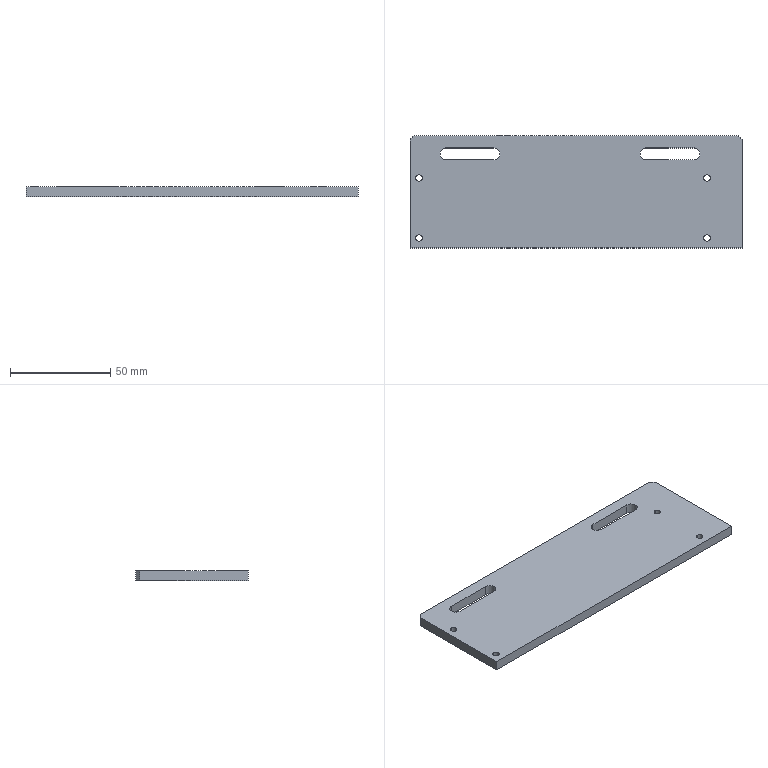Part | NX | features solid 2 | 1 solid | 24 faces | box 166 x 56 x 5 mm | volume 44572 mm3 | plane 12 | cylinder 12 | commonest cylinder face diameters 3.242 x8 6 x4
STEP:
#1=CARTESIAN_POINT('',(-350.,-1555.5,1295.));
#2=VERTEX_POINT('',#1);
#3=CARTESIAN_POINT('',(-350.,-1555.5,1300.));
#4=VERTEX_POINT('',#3);
#5=CARTESIAN_POINT('',(-350.,-1555.5,1300.));
#6=DIRECTION('',(0.,0.,1.));
#7=VECTOR('',#6,1000.);
#8=LINE('',#5,#7);
#9=EDGE_CURVE('',#2,#4,#8,.T.);
#10=ORIENTED_EDGE('',*,*,#9,.T.);
#11=CARTESIAN_POINT('',(-516.,-1555.5,1300.));
#12=VERTEX_POINT('',#11);
#13=CARTESIAN_POINT('',(-433.,-1555.5,1300.));
#14=DIRECTION('',(1.,0.,0.));
#15=VECTOR('',#14,1000.);
#16=LINE('',#13,#15);
#17=EDGE_CURVE('',#12,#4,#16,.T.);
#18=ORIENTED_EDGE('',*,*,#17,.F.);
#19=CARTESIAN_POINT('',(-516.,-1555.5,1295.));
#20=VERTEX_POINT('',#19);
#21=CARTESIAN_POINT('',(-516.,-1555.5,1300.));
#22=DIRECTION('',(0.,0.,1.));
#23=VECTOR('',#22,1000.);
#24=LINE('',#21,#23);
#25=EDGE_CURVE('',#20,#12,#24,.T.);
#26=ORIENTED_EDGE('',*,*,#25,.F.);
#27=CARTESIAN_POINT('',(-433.,-1555.5,1295.));
#28=DIRECTION('',(1.,0.,0.));
#29=VECTOR('',#28,1000.);
#30=LINE('',#27,#29);
#31=EDGE_CURVE('',#20,#2,#30,.T.);
#32=ORIENTED_EDGE('',*,*,#31,.T.);
#33=EDGE_LOOP('',(#10,#18,#26,#32));
#34=FACE_BOUND('',#33,.T.);
#35=CARTESIAN_POINT('',(-433.,-1555.5,1300.));
#36=DIRECTION('',(0.,-1.,0.));
#37=DIRECTION('',(0.,0.,-1.));
#38=AXIS2_PLACEMENT_3D('',#35,#36,#37);
#39=PLANE('',#38);
#40=ADVANCED_FACE('',(#34),#39,.T.);
#41=CARTESIAN_POINT('',(-367.5,-1518.879,1295.));
#42=VERTEX_POINT('',#41);
#43=CARTESIAN_POINT('',(-367.5,-1518.879,1300.));
#44=VERTEX_POINT('',#43);
#45=CARTESIAN_POINT('',(-367.5,-1518.879,1478.057));
#46=DIRECTION('',(0.,0.,-1.));
#47=VECTOR('',#46,1000.);
#48=LINE('',#45,#47);
#49=EDGE_CURVE('',#42,#44,#48,.F.);
#50=ORIENTED_EDGE('',*,*,#49,.T.);
#51=CARTESIAN_POINT('',(-367.5,-1522.121,1300.));
#52=VERTEX_POINT('',#51);
#53=CARTESIAN_POINT('',(-367.5,-1520.5,1300.));
#54=DIRECTION('',(0.,0.,1.));
#55=DIRECTION('',(0.,1.,0.));
#56=AXIS2_PLACEMENT_3D('',#53,#54,#55);
#57=CIRCLE('',#56,1.621);
#58=EDGE_CURVE('',#44,#52,#57,.T.);
#59=ORIENTED_EDGE('',*,*,#58,.T.);
#60=CARTESIAN_POINT('',(-367.5,-1522.121,1295.));
#61=VERTEX_POINT('',#60);
#62=CARTESIAN_POINT('',(-367.5,-1522.121,1478.057));
#63=DIRECTION('',(0.,0.,-1.));
#64=VECTOR('',#63,1000.);
#65=LINE('',#62,#64);
#66=EDGE_CURVE('',#52,#61,#65,.T.);
#67=ORIENTED_EDGE('',*,*,#66,.T.);
#68=CARTESIAN_POINT('',(-367.5,-1520.5,1295.));
#69=DIRECTION('',(0.,0.,-1.));
#70=DIRECTION('',(-1.,0.,0.));
#71=AXIS2_PLACEMENT_3D('',#68,#69,#70);
#72=CIRCLE('',#71,1.621);
#73=EDGE_CURVE('',#61,#42,#72,.T.);
#74=ORIENTED_EDGE('',*,*,#73,.T.);
#75=EDGE_LOOP('',(#50,#59,#67,#74));
#76=FACE_BOUND('',#75,.T.);
#77=CARTESIAN_POINT('',(-367.5,-1520.5,1478.057));
#78=DIRECTION('',(0.,0.,-1.));
#79=DIRECTION('',(0.,-1.,0.));
#80=AXIS2_PLACEMENT_3D('',#77,#78,#79);
#81=CYLINDRICAL_SURFACE('',#80,1.621);
#82=ADVANCED_FACE('',(#76),#81,.F.);
#83=CARTESIAN_POINT('',(-511.5,-1518.879,1295.));
#84=VERTEX_POINT('',#83);
#85=CARTESIAN_POINT('',(-511.5,-1518.879,1300.));
#86=VERTEX_POINT('',#85);
#87=CARTESIAN_POINT('',(-511.5,-1518.879,1478.057));
#88=DIRECTION('',(0.,0.,-1.));
#89=VECTOR('',#88,1000.);
#90=LINE('',#87,#89);
#91=EDGE_CURVE('',#84,#86,#90,.F.);
#92=ORIENTED_EDGE('',*,*,#91,.T.);
#93=CARTESIAN_POINT('',(-511.5,-1522.121,1300.));
#94=VERTEX_POINT('',#93);
#95=CARTESIAN_POINT('',(-511.5,-1520.5,1300.));
#96=DIRECTION('',(0.,0.,1.));
#97=DIRECTION('',(0.,1.,0.));
#98=AXIS2_PLACEMENT_3D('',#95,#96,#97);
#99=CIRCLE('',#98,1.621);
#100=EDGE_CURVE('',#86,#94,#99,.T.);
#101=ORIENTED_EDGE('',*,*,#100,.T.);
#102=CARTESIAN_POINT('',(-511.5,-1522.121,1295.));
#103=VERTEX_POINT('',#102);
#104=CARTESIAN_POINT('',(-511.5,-1522.121,1478.057));
#105=DIRECTION('',(0.,0.,-1.));
#106=VECTOR('',#105,1000.);
#107=LINE('',#104,#106);
#108=EDGE_CURVE('',#94,#103,#107,.T.);
#109=ORIENTED_EDGE('',*,*,#108,.T.);
#110=CARTESIAN_POINT('',(-511.5,-1520.5,1295.));
#111=DIRECTION('',(0.,0.,-1.));
#112=DIRECTION('',(-1.,0.,0.));
#113=AXIS2_PLACEMENT_3D('',#110,#111,#112);
#114=CIRCLE('',#113,1.621);
#115=EDGE_CURVE('',#103,#84,#114,.T.);
#116=ORIENTED_EDGE('',*,*,#115,.T.);
#117=EDGE_LOOP('',(#92,#101,#109,#116));
#118=FACE_BOUND('',#117,.T.);
#119=CARTESIAN_POINT('',(-511.5,-1520.5,1478.057));
#120=DIRECTION('',(0.,0.,-1.));
#121=DIRECTION('',(0.,-1.,0.));
#122=AXIS2_PLACEMENT_3D('',#119,#120,#121);
#123=CYLINDRICAL_SURFACE('',#122,1.621);
#124=ADVANCED_FACE('',(#118),#123,.F.);
#125=CARTESIAN_POINT('',(-511.5,-1548.879,1300.));
#126=VERTEX_POINT('',#125);
#127=CARTESIAN_POINT('',(-511.5,-1548.879,1295.));
#128=VERTEX_POINT('',#127);
#129=CARTESIAN_POINT('',(-511.5,-1548.879,1478.057));
#130=DIRECTION('',(0.,0.,-1.));
#131=VECTOR('',#130,1000.);
#132=LINE('',#129,#131);
#133=EDGE_CURVE('',#126,#128,#132,.T.);
#134=ORIENTED_EDGE('',*,*,#133,.F.);
#135=CARTESIAN_POINT('',(-511.5,-1552.121,1300.));
#136=VERTEX_POINT('',#135);
#137=CARTESIAN_POINT('',(-511.5,-1550.5,1300.));
#138=DIRECTION('',(0.,0.,1.));
#139=DIRECTION('',(0.,1.,0.));
#140=AXIS2_PLACEMENT_3D('',#137,#138,#139);
#141=CIRCLE('',#140,1.621);
#142=EDGE_CURVE('',#126,#136,#141,.T.);
#143=ORIENTED_EDGE('',*,*,#142,.T.);
#144=CARTESIAN_POINT('',(-511.5,-1552.121,1295.));
#145=VERTEX_POINT('',#144);
#146=CARTESIAN_POINT('',(-511.5,-1552.121,1478.057));
#147=DIRECTION('',(0.,0.,-1.));
#148=VECTOR('',#147,1000.);
#149=LINE('',#146,#148);
#150=EDGE_CURVE('',#145,#136,#149,.F.);
#151=ORIENTED_EDGE('',*,*,#150,.F.);
#152=CARTESIAN_POINT('',(-511.5,-1550.5,1295.));
#153=DIRECTION('',(0.,0.,-1.));
#154=DIRECTION('',(-1.,0.,0.));
#155=AXIS2_PLACEMENT_3D('',#152,#153,#154);
#156=CIRCLE('',#155,1.621);
#157=EDGE_CURVE('',#145,#128,#156,.T.);
#158=ORIENTED_EDGE('',*,*,#157,.T.);
#159=EDGE_LOOP('',(#134,#143,#151,#158));
#160=FACE_BOUND('',#159,.T.);
#161=CARTESIAN_POINT('',(-511.5,-1550.5,1478.057));
#162=DIRECTION('',(0.,0.,-1.));
#163=DIRECTION('',(0.,-1.,0.));
#164=AXIS2_PLACEMENT_3D('',#161,#162,#163);
#165=CYLINDRICAL_SURFACE('',#164,1.621);
#166=ADVANCED_FACE('',(#160),#165,.F.);
#167=CARTESIAN_POINT('',(-367.5,-1548.879,1300.));
#168=VERTEX_POINT('',#167);
#169=CARTESIAN_POINT('',(-367.5,-1548.879,1295.));
#170=VERTEX_POINT('',#169);
#171=CARTESIAN_POINT('',(-367.5,-1548.879,1478.057));
#172=DIRECTION('',(0.,0.,-1.));
#173=VECTOR('',#172,1000.);
#174=LINE('',#171,#173);
#175=EDGE_CURVE('',#168,#170,#174,.T.);
#176=ORIENTED_EDGE('',*,*,#175,.F.);
#177=CARTESIAN_POINT('',(-367.5,-1552.121,1300.));
#178=VERTEX_POINT('',#177);
#179=CARTESIAN_POINT('',(-367.5,-1550.5,1300.));
#180=DIRECTION('',(0.,0.,1.));
#181=DIRECTION('',(0.,1.,0.));
#182=AXIS2_PLACEMENT_3D('',#179,#180,#181);
#183=CIRCLE('',#182,1.621);
#184=EDGE_CURVE('',#168,#178,#183,.T.);
#185=ORIENTED_EDGE('',*,*,#184,.T.);
#186=CARTESIAN_POINT('',(-367.5,-1552.121,1295.));
#187=VERTEX_POINT('',#186);
#188=CARTESIAN_POINT('',(-367.5,-1552.121,1478.057));
#189=DIRECTION('',(0.,0.,-1.));
#190=VECTOR('',#189,1000.);
#191=LINE('',#188,#190);
#192=EDGE_CURVE('',#187,#178,#191,.F.);
#193=ORIENTED_EDGE('',*,*,#192,.F.);
#194=CARTESIAN_POINT('',(-367.5,-1550.5,1295.));
#195=DIRECTION('',(0.,0.,-1.));
#196=DIRECTION('',(-1.,0.,0.));
#197=AXIS2_PLACEMENT_3D('',#194,#195,#196);
#198=CIRCLE('',#197,1.621);
#199=EDGE_CURVE('',#187,#170,#198,.T.);
#200=ORIENTED_EDGE('',*,*,#199,.T.);
#201=EDGE_LOOP('',(#176,#185,#193,#200));
#202=FACE_BOUND('',#201,.T.);
#203=CARTESIAN_POINT('',(-367.5,-1550.5,1478.057));
#204=DIRECTION('',(0.,0.,-1.));
#205=DIRECTION('',(0.,-1.,0.));
#206=AXIS2_PLACEMENT_3D('',#203,#204,#205);
#207=CYLINDRICAL_SURFACE('',#206,1.621);
#208=ADVANCED_FACE('',(#202),#207,.F.);
#209=CARTESIAN_POINT('',(-398.,-1511.5,1300.));
#210=VERTEX_POINT('',#209);
#211=CARTESIAN_POINT('',(-374.,-1511.5,1300.));
#212=VERTEX_POINT('',#211);
#213=CARTESIAN_POINT('',(-433.,-1511.5,1300.));
#214=DIRECTION('',(1.,0.,0.));
#215=VECTOR('',#214,1000.);
#216=LINE('',#213,#215);
#217=EDGE_CURVE('',#210,#212,#216,.T.);
#218=ORIENTED_EDGE('',*,*,#217,.T.);
#219=CARTESIAN_POINT('',(-374.,-1511.5,1295.));
#220=VERTEX_POINT('',#219);
#221=CARTESIAN_POINT('',(-374.,-1511.5,1478.057));
#222=DIRECTION('',(0.,0.,-1.));
#223=VECTOR('',#222,1000.);
#224=LINE('',#221,#223);
#225=EDGE_CURVE('',#212,#220,#224,.T.);
#226=ORIENTED_EDGE('',*,*,#225,.T.);
#227=CARTESIAN_POINT('',(-398.,-1511.5,1295.));
#228=VERTEX_POINT('',#227);
#229=CARTESIAN_POINT('',(-374.,-1511.5,1295.));
#230=DIRECTION('',(-1.,0.,0.));
#231=VECTOR('',#230,1000.);
#232=LINE('',#229,#231);
#233=EDGE_CURVE('',#220,#228,#232,.T.);
#234=ORIENTED_EDGE('',*,*,#233,.T.);
#235=CARTESIAN_POINT('',(-398.,-1511.5,1478.057));
#236=DIRECTION('',(0.,0.,-1.));
#237=VECTOR('',#236,1000.);
#238=LINE('',#235,#237);
#239=EDGE_CURVE('',#210,#228,#238,.T.);
#240=ORIENTED_EDGE('',*,*,#239,.F.);
#241=EDGE_LOOP('',(#218,#226,#234,#240));
#242=FACE_BOUND('',#241,.T.);
#243=CARTESIAN_POINT('',(-374.,-1511.5,1478.057));
#244=DIRECTION('',(0.,-1.,0.));
#245=DIRECTION('',(0.,0.,-1.));
#246=AXIS2_PLACEMENT_3D('',#243,#244,#245);
#247=PLANE('',#246);
#248=ADVANCED_FACE('',(#242),#247,.F.);
#249=CARTESIAN_POINT('',(-374.,-1505.5,1300.));
#250=VERTEX_POINT('',#249);
#251=CARTESIAN_POINT('',(-374.,-1508.5,1300.));
#252=DIRECTION('',(0.,0.,1.));
#253=DIRECTION('',(0.,1.,0.));
#254=AXIS2_PLACEMENT_3D('',#251,#252,#253);
#255=CIRCLE('',#254,3.);
#256=EDGE_CURVE('',#212,#250,#255,.T.);
#257=ORIENTED_EDGE('',*,*,#256,.T.);
#258=CARTESIAN_POINT('',(-374.,-1505.5,1295.));
#259=VERTEX_POINT('',#258);
#260=CARTESIAN_POINT('',(-374.,-1505.5,1478.057));
#261=DIRECTION('',(0.,0.,-1.));
#262=VECTOR('',#261,1000.);
#263=LINE('',#260,#262);
#264=EDGE_CURVE('',#250,#259,#263,.T.);
#265=ORIENTED_EDGE('',*,*,#264,.T.);
#266=CARTESIAN_POINT('',(-374.,-1508.5,1295.));
#267=DIRECTION('',(0.,0.,-1.));
#268=DIRECTION('',(-1.,0.,0.));
#269=AXIS2_PLACEMENT_3D('',#266,#267,#268);
#270=CIRCLE('',#269,3.);
#271=EDGE_CURVE('',#259,#220,#270,.T.);
#272=ORIENTED_EDGE('',*,*,#271,.T.);
#273=ORIENTED_EDGE('',*,*,#225,.F.);
#274=EDGE_LOOP('',(#257,#265,#272,#273));
#275=FACE_BOUND('',#274,.T.);
#276=CARTESIAN_POINT('',(-374.,-1508.5,1478.057));
#277=DIRECTION('',(0.,0.,-1.));
#278=DIRECTION('',(0.,-1.,0.));
#279=AXIS2_PLACEMENT_3D('',#276,#277,#278);
#280=CYLINDRICAL_SURFACE('',#279,3.);
#281=ADVANCED_FACE('',(#275),#280,.F.);
#282=CARTESIAN_POINT('',(-398.,-1505.5,1300.));
#283=VERTEX_POINT('',#282);
#284=CARTESIAN_POINT('',(-433.,-1505.5,1300.));
#285=DIRECTION('',(-1.,0.,0.));
#286=VECTOR('',#285,1000.);
#287=LINE('',#284,#286);
#288=EDGE_CURVE('',#250,#283,#287,.T.);
#289=ORIENTED_EDGE('',*,*,#288,.T.);
#290=CARTESIAN_POINT('',(-398.,-1505.5,1295.));
#291=VERTEX_POINT('',#290);
#292=CARTESIAN_POINT('',(-398.,-1505.5,1478.057));
#293=DIRECTION('',(0.,0.,-1.));
#294=VECTOR('',#293,1000.);
#295=LINE('',#292,#294);
#296=EDGE_CURVE('',#283,#291,#295,.T.);
#297=ORIENTED_EDGE('',*,*,#296,.T.);
#298=CARTESIAN_POINT('',(-374.,-1505.5,1295.));
#299=DIRECTION('',(1.,0.,0.));
#300=VECTOR('',#299,1000.);
#301=LINE('',#298,#300);
#302=EDGE_CURVE('',#291,#259,#301,.T.);
#303=ORIENTED_EDGE('',*,*,#302,.T.);
#304=ORIENTED_EDGE('',*,*,#264,.F.);
#305=EDGE_LOOP('',(#289,#297,#303,#304));
#306=FACE_BOUND('',#305,.T.);
#307=CARTESIAN_POINT('',(-374.,-1505.5,1478.057));
#308=DIRECTION('',(0.,1.,0.));
#309=DIRECTION('',(1.,0.,0.));
#310=AXIS2_PLACEMENT_3D('',#307,#308,#309);
#311=PLANE('',#310);
#312=ADVANCED_FACE('',(#306),#311,.F.);
#313=CARTESIAN_POINT('',(-398.,-1508.5,1300.));
#314=DIRECTION('',(0.,0.,1.));
#315=DIRECTION('',(0.,1.,0.));
#316=AXIS2_PLACEMENT_3D('',#313,#314,#315);
#317=CIRCLE('',#316,3.);
#318=EDGE_CURVE('',#283,#210,#317,.T.);
#319=ORIENTED_EDGE('',*,*,#318,.T.);
#320=ORIENTED_EDGE('',*,*,#239,.T.);
#321=CARTESIAN_POINT('',(-398.,-1508.5,1295.));
#322=DIRECTION('',(0.,0.,-1.));
#323=DIRECTION('',(1.,0.,0.));
#324=AXIS2_PLACEMENT_3D('',#321,#322,#323);
#325=CIRCLE('',#324,3.);
#326=EDGE_CURVE('',#228,#291,#325,.T.);
#327=ORIENTED_EDGE('',*,*,#326,.T.);
#328=ORIENTED_EDGE('',*,*,#296,.F.);
#329=EDGE_LOOP('',(#319,#320,#327,#328));
#330=FACE_BOUND('',#329,.T.);
#331=CARTESIAN_POINT('',(-398.,-1508.5,1478.057));
#332=DIRECTION('',(0.,0.,-1.));
#333=DIRECTION('',(0.,-1.,0.));
#334=AXIS2_PLACEMENT_3D('',#331,#332,#333);
#335=CYLINDRICAL_SURFACE('',#334,3.);
#336=ADVANCED_FACE('',(#330),#335,.F.);
#337=CARTESIAN_POINT('',(-498.,-1511.5,1300.));
#338=VERTEX_POINT('',#337);
#339=CARTESIAN_POINT('',(-474.,-1511.5,1300.));
#340=VERTEX_POINT('',#339);
#341=CARTESIAN_POINT('',(-433.,-1511.5,1300.));
#342=DIRECTION('',(1.,0.,0.));
#343=VECTOR('',#342,1000.);
#344=LINE('',#341,#343);
#345=EDGE_CURVE('',#338,#340,#344,.T.);
#346=ORIENTED_EDGE('',*,*,#345,.T.);
#347=CARTESIAN_POINT('',(-474.,-1511.5,1295.));
#348=VERTEX_POINT('',#347);
#349=CARTESIAN_POINT('',(-474.,-1511.5,1478.057));
#350=DIRECTION('',(0.,0.,-1.));
#351=VECTOR('',#350,1000.);
#352=LINE('',#349,#351);
#353=EDGE_CURVE('',#340,#348,#352,.T.);
#354=ORIENTED_EDGE('',*,*,#353,.T.);
#355=CARTESIAN_POINT('',(-498.,-1511.5,1295.));
#356=VERTEX_POINT('',#355);
#357=CARTESIAN_POINT('',(-474.,-1511.5,1295.));
#358=DIRECTION('',(-1.,0.,0.));
#359=VECTOR('',#358,1000.);
#360=LINE('',#357,#359);
#361=EDGE_CURVE('',#348,#356,#360,.T.);
#362=ORIENTED_EDGE('',*,*,#361,.T.);
#363=CARTESIAN_POINT('',(-498.,-1511.5,1478.057));
#364=DIRECTION('',(0.,0.,-1.));
#365=VECTOR('',#364,1000.);
#366=LINE('',#363,#365);
#367=EDGE_CURVE('',#338,#356,#366,.T.);
#368=ORIENTED_EDGE('',*,*,#367,.F.);
#369=EDGE_LOOP('',(#346,#354,#362,#368));
#370=FACE_BOUND('',#369,.T.);
#371=CARTESIAN_POINT('',(-474.,-1511.5,1478.057));
#372=DIRECTION('',(0.,-1.,0.));
#373=DIRECTION('',(0.,0.,-1.));
#374=AXIS2_PLACEMENT_3D('',#371,#372,#373);
#375=PLANE('',#374);
#376=ADVANCED_FACE('',(#370),#375,.F.);
#377=CARTESIAN_POINT('',(-474.,-1505.5,1300.));
#378=VERTEX_POINT('',#377);
#379=CARTESIAN_POINT('',(-474.,-1508.5,1300.));
#380=DIRECTION('',(0.,0.,1.));
#381=DIRECTION('',(0.,1.,0.));
#382=AXIS2_PLACEMENT_3D('',#379,#380,#381);
#383=CIRCLE('',#382,3.);
#384=EDGE_CURVE('',#340,#378,#383,.T.);
#385=ORIENTED_EDGE('',*,*,#384,.T.);
#386=CARTESIAN_POINT('',(-474.,-1505.5,1295.));
#387=VERTEX_POINT('',#386);
#388=CARTESIAN_POINT('',(-474.,-1505.5,1478.057));
#389=DIRECTION('',(0.,0.,-1.));
#390=VECTOR('',#389,1000.);
#391=LINE('',#388,#390);
#392=EDGE_CURVE('',#378,#387,#391,.T.);
#393=ORIENTED_EDGE('',*,*,#392,.T.);
#394=CARTESIAN_POINT('',(-474.,-1508.5,1295.));
#395=DIRECTION('',(0.,0.,-1.));
#396=DIRECTION('',(-1.,0.,0.));
#397=AXIS2_PLACEMENT_3D('',#394,#395,#396);
#398=CIRCLE('',#397,3.);
#399=EDGE_CURVE('',#387,#348,#398,.T.);
#400=ORIENTED_EDGE('',*,*,#399,.T.);
#401=ORIENTED_EDGE('',*,*,#353,.F.);
#402=EDGE_LOOP('',(#385,#393,#400,#401));
#403=FACE_BOUND('',#402,.T.);
#404=CARTESIAN_POINT('',(-474.,-1508.5,1478.057));
#405=DIRECTION('',(0.,0.,-1.));
#406=DIRECTION('',(0.,-1.,0.));
#407=AXIS2_PLACEMENT_3D('',#404,#405,#406);
#408=CYLINDRICAL_SURFACE('',#407,3.);
#409=ADVANCED_FACE('',(#403),#408,.F.);
#410=CARTESIAN_POINT('',(-498.,-1505.5,1300.));
#411=VERTEX_POINT('',#410);
#412=CARTESIAN_POINT('',(-433.,-1505.5,1300.));
#413=DIRECTION('',(-1.,0.,0.));
#414=VECTOR('',#413,1000.);
#415=LINE('',#412,#414);
#416=EDGE_CURVE('',#378,#411,#415,.T.);
#417=ORIENTED_EDGE('',*,*,#416,.T.);
#418=CARTESIAN_POINT('',(-498.,-1505.5,1295.));
#419=VERTEX_POINT('',#418);
#420=CARTESIAN_POINT('',(-498.,-1505.5,1478.057));
#421=DIRECTION('',(0.,0.,-1.));
#422=VECTOR('',#421,1000.);
#423=LINE('',#420,#422);
#424=EDGE_CURVE('',#411,#419,#423,.T.);
#425=ORIENTED_EDGE('',*,*,#424,.T.);
#426=CARTESIAN_POINT('',(-474.,-1505.5,1295.));
#427=DIRECTION('',(1.,0.,0.));
#428=VECTOR('',#427,1000.);
#429=LINE('',#426,#428);
#430=EDGE_CURVE('',#419,#387,#429,.T.);
#431=ORIENTED_EDGE('',*,*,#430,.T.);
#432=ORIENTED_EDGE('',*,*,#392,.F.);
#433=EDGE_LOOP('',(#417,#425,#431,#432));
#434=FACE_BOUND('',#433,.T.);
#435=CARTESIAN_POINT('',(-474.,-1505.5,1478.057));
#436=DIRECTION('',(0.,1.,0.));
#437=DIRECTION('',(1.,0.,0.));
#438=AXIS2_PLACEMENT_3D('',#435,#436,#437);
#439=PLANE('',#438);
#440=ADVANCED_FACE('',(#434),#439,.F.);
#441=CARTESIAN_POINT('',(-498.,-1508.5,1300.));
#442=DIRECTION('',(0.,0.,1.));
#443=DIRECTION('',(0.,1.,0.));
#444=AXIS2_PLACEMENT_3D('',#441,#442,#443);
#445=CIRCLE('',#444,3.);
#446=EDGE_CURVE('',#411,#338,#445,.T.);
#447=ORIENTED_EDGE('',*,*,#446,.T.);
#448=ORIENTED_EDGE('',*,*,#367,.T.);
#449=CARTESIAN_POINT('',(-498.,-1508.5,1295.));
#450=DIRECTION('',(0.,0.,-1.));
#451=DIRECTION('',(1.,0.,0.));
#452=AXIS2_PLACEMENT_3D('',#449,#450,#451);
#453=CIRCLE('',#452,3.);
#454=EDGE_CURVE('',#356,#419,#453,.T.);
#455=ORIENTED_EDGE('',*,*,#454,.T.);
#456=ORIENTED_EDGE('',*,*,#424,.F.);
#457=EDGE_LOOP('',(#447,#448,#455,#456));
#458=FACE_BOUND('',#457,.T.);
#459=CARTESIAN_POINT('',(-498.,-1508.5,1478.057));
#460=DIRECTION('',(0.,0.,-1.));
#461=DIRECTION('',(0.,-1.,0.));
#462=AXIS2_PLACEMENT_3D('',#459,#460,#461);
#463=CYLINDRICAL_SURFACE('',#462,3.);
#464=ADVANCED_FACE('',(#458),#463,.F.);
#465=ORIENTED_EDGE('',*,*,#446,.F.);
#466=ORIENTED_EDGE('',*,*,#416,.F.);
#467=ORIENTED_EDGE('',*,*,#384,.F.);
#468=ORIENTED_EDGE('',*,*,#345,.F.);
#469=EDGE_LOOP('',(#465,#466,#467,#468));
#470=FACE_BOUND('',#469,.T.);
#471=ORIENTED_EDGE('',*,*,#318,.F.);
#472=ORIENTED_EDGE('',*,*,#288,.F.);
#473=ORIENTED_EDGE('',*,*,#256,.F.);
#474=ORIENTED_EDGE('',*,*,#217,.F.);
#475=EDGE_LOOP('',(#471,#472,#473,#474));
#476=FACE_BOUND('',#475,.T.);
#477=CARTESIAN_POINT('',(-367.5,-1550.5,1300.));
#478=DIRECTION('',(0.,0.,1.));
#479=DIRECTION('',(0.,1.,0.));
#480=AXIS2_PLACEMENT_3D('',#477,#478,#479);
#481=CIRCLE('',#480,1.621);
#482=EDGE_CURVE('',#178,#168,#481,.T.);
#483=ORIENTED_EDGE('',*,*,#482,.F.);
#484=ORIENTED_EDGE('',*,*,#184,.F.);
#485=EDGE_LOOP('',(#483,#484));
#486=FACE_BOUND('',#485,.T.);
#487=CARTESIAN_POINT('',(-511.5,-1550.5,1300.));
#488=DIRECTION('',(0.,0.,1.));
#489=DIRECTION('',(0.,1.,0.));
#490=AXIS2_PLACEMENT_3D('',#487,#488,#489);
#491=CIRCLE('',#490,1.621);
#492=EDGE_CURVE('',#136,#126,#491,.T.);
#493=ORIENTED_EDGE('',*,*,#492,.F.);
#494=ORIENTED_EDGE('',*,*,#142,.F.);
#495=EDGE_LOOP('',(#493,#494));
#496=FACE_BOUND('',#495,.T.);
#497=CARTESIAN_POINT('',(-511.5,-1520.5,1300.));
#498=DIRECTION('',(0.,0.,1.));
#499=DIRECTION('',(0.,1.,0.));
#500=AXIS2_PLACEMENT_3D('',#497,#498,#499);
#501=CIRCLE('',#500,1.621);
#502=EDGE_CURVE('',#94,#86,#501,.T.);
#503=ORIENTED_EDGE('',*,*,#502,.F.);
#504=ORIENTED_EDGE('',*,*,#100,.F.);
#505=EDGE_LOOP('',(#503,#504));
#506=FACE_BOUND('',#505,.T.);
#507=CARTESIAN_POINT('',(-367.5,-1520.5,1300.));
#508=DIRECTION('',(0.,0.,1.));
#509=DIRECTION('',(0.,1.,0.));
#510=AXIS2_PLACEMENT_3D('',#507,#508,#509);
#511=CIRCLE('',#510,1.621);
#512=EDGE_CURVE('',#52,#44,#511,.T.);
#513=ORIENTED_EDGE('',*,*,#512,.F.);
#514=ORIENTED_EDGE('',*,*,#58,.F.);
#515=EDGE_LOOP('',(#513,#514));
#516=FACE_BOUND('',#515,.T.);
#517=ORIENTED_EDGE('',*,*,#17,.T.);
#518=CARTESIAN_POINT('',(-350.,-1501.5,1300.));
#519=VERTEX_POINT('',#518);
#520=CARTESIAN_POINT('',(-350.,-1569.5,1300.));
#521=DIRECTION('',(0.,1.,0.));
#522=VECTOR('',#521,1000.);
#523=LINE('',#520,#522);
#524=EDGE_CURVE('',#4,#519,#523,.T.);
#525=ORIENTED_EDGE('',*,*,#524,.T.);
#526=CARTESIAN_POINT('',(-352.,-1499.5,1300.));
#527=VERTEX_POINT('',#526);
#528=CARTESIAN_POINT('',(-352.,-1499.5,1300.));
#529=DIRECTION('',(-0.7071,0.7071,0.));
#530=VECTOR('',#529,1000.);
#531=LINE('',#528,#530);
#532=EDGE_CURVE('',#519,#527,#531,.T.);
#533=ORIENTED_EDGE('',*,*,#532,.T.);
#534=CARTESIAN_POINT('',(-514.,-1499.5,1300.));
#535=VERTEX_POINT('',#534);
#536=CARTESIAN_POINT('',(-352.,-1499.5,1300.));
#537=DIRECTION('',(-1.,0.,0.));
#538=VECTOR('',#537,1000.);
#539=LINE('',#536,#538);
#540=EDGE_CURVE('',#527,#535,#539,.T.);
#541=ORIENTED_EDGE('',*,*,#540,.T.);
#542=CARTESIAN_POINT('',(-516.,-1501.5,1300.));
#543=VERTEX_POINT('',#542);
#544=CARTESIAN_POINT('',(-514.,-1499.5,1300.));
#545=DIRECTION('',(-0.7071,-0.7071,0.));
#546=VECTOR('',#545,1000.);
#547=LINE('',#544,#546);
#548=EDGE_CURVE('',#535,#543,#547,.T.);
#549=ORIENTED_EDGE('',*,*,#548,.T.);
#550=CARTESIAN_POINT('',(-516.,-1501.5,1300.));
#551=DIRECTION('',(0.,-1.,0.));
#552=VECTOR('',#551,1000.);
#553=LINE('',#550,#552);
#554=EDGE_CURVE('',#543,#12,#553,.T.);
#555=ORIENTED_EDGE('',*,*,#554,.T.);
#556=EDGE_LOOP('',(#517,#525,#533,#541,#549,#555));
#557=FACE_BOUND('',#556,.T.);
#558=CARTESIAN_POINT('',(-433.,-1418.5,1300.));
#559=DIRECTION('',(0.,0.,1.));
#560=DIRECTION('',(0.,-1.,0.));
#561=AXIS2_PLACEMENT_3D('',#558,#559,#560);
#562=PLANE('',#561);
#563=ADVANCED_FACE('',(#470,#476,#486,#496,#506,#516,#557),#562,.T.);
#564=ORIENTED_EDGE('',*,*,#430,.F.);
#565=ORIENTED_EDGE('',*,*,#454,.F.);
#566=ORIENTED_EDGE('',*,*,#361,.F.);
#567=ORIENTED_EDGE('',*,*,#399,.F.);
#568=EDGE_LOOP('',(#564,#565,#566,#567));
#569=FACE_BOUND('',#568,.T.);
#570=ORIENTED_EDGE('',*,*,#302,.F.);
#571=ORIENTED_EDGE('',*,*,#326,.F.);
#572=ORIENTED_EDGE('',*,*,#233,.F.);
#573=ORIENTED_EDGE('',*,*,#271,.F.);
#574=EDGE_LOOP('',(#570,#571,#572,#573));
#575=FACE_BOUND('',#574,.T.);
#576=ORIENTED_EDGE('',*,*,#199,.F.);
#577=CARTESIAN_POINT('',(-367.5,-1550.5,1295.));
#578=DIRECTION('',(0.,0.,-1.));
#579=DIRECTION('',(-1.,0.,0.));
#580=AXIS2_PLACEMENT_3D('',#577,#578,#579);
#581=CIRCLE('',#580,1.621);
#582=EDGE_CURVE('',#170,#187,#581,.T.);
#583=ORIENTED_EDGE('',*,*,#582,.F.);
#584=EDGE_LOOP('',(#576,#583));
#585=FACE_BOUND('',#584,.T.);
#586=ORIENTED_EDGE('',*,*,#157,.F.);
#587=CARTESIAN_POINT('',(-511.5,-1550.5,1295.));
#588=DIRECTION('',(0.,0.,-1.));
#589=DIRECTION('',(-1.,0.,0.));
#590=AXIS2_PLACEMENT_3D('',#587,#588,#589);
#591=CIRCLE('',#590,1.621);
#592=EDGE_CURVE('',#128,#145,#591,.T.);
#593=ORIENTED_EDGE('',*,*,#592,.F.);
#594=EDGE_LOOP('',(#586,#593));
#595=FACE_BOUND('',#594,.T.);
#596=ORIENTED_EDGE('',*,*,#115,.F.);
#597=CARTESIAN_POINT('',(-511.5,-1520.5,1295.));
#598=DIRECTION('',(0.,0.,-1.));
#599=DIRECTION('',(-1.,0.,0.));
#600=AXIS2_PLACEMENT_3D('',#597,#598,#599);
#601=CIRCLE('',#600,1.621);
#602=EDGE_CURVE('',#84,#103,#601,.T.);
#603=ORIENTED_EDGE('',*,*,#602,.F.);
#604=EDGE_LOOP('',(#596,#603));
#605=FACE_BOUND('',#604,.T.);
#606=ORIENTED_EDGE('',*,*,#73,.F.);
#607=CARTESIAN_POINT('',(-367.5,-1520.5,1295.));
#608=DIRECTION('',(0.,0.,-1.));
#609=DIRECTION('',(-1.,0.,0.));
#610=AXIS2_PLACEMENT_3D('',#607,#608,#609);
#611=CIRCLE('',#610,1.621);
#612=EDGE_CURVE('',#42,#61,#611,.T.);
#613=ORIENTED_EDGE('',*,*,#612,.F.);
#614=EDGE_LOOP('',(#606,#613));
#615=FACE_BOUND('',#614,.T.);
#616=CARTESIAN_POINT('',(-350.,-1501.5,1295.));
#617=VERTEX_POINT('',#616);
#618=CARTESIAN_POINT('',(-350.,-1569.5,1295.));
#619=DIRECTION('',(0.,1.,0.));
#620=VECTOR('',#619,1000.);
#621=LINE('',#618,#620);
#622=EDGE_CURVE('',#2,#617,#621,.T.);
#623=ORIENTED_EDGE('',*,*,#622,.F.);
#624=ORIENTED_EDGE('',*,*,#31,.F.);
#625=CARTESIAN_POINT('',(-516.,-1501.5,1295.));
#626=VERTEX_POINT('',#625);
#627=CARTESIAN_POINT('',(-516.,-1501.5,1295.));
#628=DIRECTION('',(0.,-1.,0.));
#629=VECTOR('',#628,1000.);
#630=LINE('',#627,#629);
#631=EDGE_CURVE('',#626,#20,#630,.T.);
#632=ORIENTED_EDGE('',*,*,#631,.F.);
#633=CARTESIAN_POINT('',(-514.,-1499.5,1295.));
#634=VERTEX_POINT('',#633);
#635=CARTESIAN_POINT('',(-514.,-1499.5,1295.));
#636=DIRECTION('',(-0.7071,-0.7071,0.));
#637=VECTOR('',#636,1000.);
#638=LINE('',#635,#637);
#639=EDGE_CURVE('',#634,#626,#638,.T.);
#640=ORIENTED_EDGE('',*,*,#639,.F.);
#641=CARTESIAN_POINT('',(-352.,-1499.5,1295.));
#642=VERTEX_POINT('',#641);
#643=CARTESIAN_POINT('',(-352.,-1499.5,1295.));
#644=DIRECTION('',(-1.,0.,0.));
#645=VECTOR('',#644,1000.);
#646=LINE('',#643,#645);
#647=EDGE_CURVE('',#642,#634,#646,.T.);
#648=ORIENTED_EDGE('',*,*,#647,.F.);
#649=CARTESIAN_POINT('',(-352.,-1499.5,1295.));
#650=DIRECTION('',(-0.7071,0.7071,0.));
#651=VECTOR('',#650,1000.);
#652=LINE('',#649,#651);
#653=EDGE_CURVE('',#617,#642,#652,.T.);
#654=ORIENTED_EDGE('',*,*,#653,.F.);
#655=EDGE_LOOP('',(#623,#624,#632,#640,#648,#654));
#656=FACE_BOUND('',#655,.T.);
#657=CARTESIAN_POINT('',(-433.,-1418.5,1295.));
#658=DIRECTION('',(0.,0.,1.));
#659=DIRECTION('',(0.,-1.,0.));
#660=AXIS2_PLACEMENT_3D('',#657,#658,#659);
#661=PLANE('',#660);
#662=ADVANCED_FACE('',(#569,#575,#585,#595,#605,#615,#656),#661,.F.);
#663=ORIENTED_EDGE('',*,*,#9,.F.);
#664=ORIENTED_EDGE('',*,*,#622,.T.);
#665=CARTESIAN_POINT('',(-350.,-1501.5,1295.));
#666=DIRECTION('',(0.,0.,1.));
#667=VECTOR('',#666,1000.);
#668=LINE('',#665,#667);
#669=EDGE_CURVE('',#617,#519,#668,.T.);
#670=ORIENTED_EDGE('',*,*,#669,.T.);
#671=ORIENTED_EDGE('',*,*,#524,.F.);
#672=EDGE_LOOP('',(#663,#664,#670,#671));
#673=FACE_BOUND('',#672,.T.);
#674=CARTESIAN_POINT('',(-350.,-1569.5,1295.));
#675=DIRECTION('',(1.,0.,0.));
#676=DIRECTION('',(0.,1.,0.));
#677=AXIS2_PLACEMENT_3D('',#674,#675,#676);
#678=PLANE('',#677);
#679=ADVANCED_FACE('',(#673),#678,.T.);
#680=ORIENTED_EDGE('',*,*,#25,.T.);
#681=ORIENTED_EDGE('',*,*,#554,.F.);
#682=CARTESIAN_POINT('',(-516.,-1501.5,1295.));
#683=DIRECTION('',(0.,0.,1.));
#684=VECTOR('',#683,1000.);
#685=LINE('',#682,#684);
#686=EDGE_CURVE('',#626,#543,#685,.T.);
#687=ORIENTED_EDGE('',*,*,#686,.F.);
#688=ORIENTED_EDGE('',*,*,#631,.T.);
#689=EDGE_LOOP('',(#680,#681,#687,#688));
#690=FACE_BOUND('',#689,.T.);
#691=CARTESIAN_POINT('',(-516.,-1501.5,1295.));
#692=DIRECTION('',(-1.,0.,0.));
#693=DIRECTION('',(0.,1.,0.));
#694=AXIS2_PLACEMENT_3D('',#691,#692,#693);
#695=PLANE('',#694);
#696=ADVANCED_FACE('',(#690),#695,.T.);
#697=ORIENTED_EDGE('',*,*,#548,.F.);
#698=CARTESIAN_POINT('',(-514.,-1499.5,1295.));
#699=DIRECTION('',(0.,0.,1.));
#700=VECTOR('',#699,1000.);
#701=LINE('',#698,#700);
#702=EDGE_CURVE('',#634,#535,#701,.T.);
#703=ORIENTED_EDGE('',*,*,#702,.F.);
#704=ORIENTED_EDGE('',*,*,#639,.T.);
#705=ORIENTED_EDGE('',*,*,#686,.T.);
#706=EDGE_LOOP('',(#697,#703,#704,#705));
#707=FACE_BOUND('',#706,.T.);
#708=CARTESIAN_POINT('',(-514.,-1499.5,1295.));
#709=DIRECTION('',(-0.7071,0.7071,0.));
#710=DIRECTION('',(0.,0.,1.));
#711=AXIS2_PLACEMENT_3D('',#708,#709,#710);
#712=PLANE('',#711);
#713=ADVANCED_FACE('',(#707),#712,.T.);
#714=ORIENTED_EDGE('',*,*,#540,.F.);
#715=CARTESIAN_POINT('',(-352.,-1499.5,1295.));
#716=DIRECTION('',(0.,0.,1.));
#717=VECTOR('',#716,1000.);
#718=LINE('',#715,#717);
#719=EDGE_CURVE('',#642,#527,#718,.T.);
#720=ORIENTED_EDGE('',*,*,#719,.F.);
#721=ORIENTED_EDGE('',*,*,#647,.T.);
#722=ORIENTED_EDGE('',*,*,#702,.T.);
#723=EDGE_LOOP('',(#714,#720,#721,#722));
#724=FACE_BOUND('',#723,.T.);
#725=CARTESIAN_POINT('',(-352.,-1499.5,1295.));
#726=DIRECTION('',(0.,1.,0.));
#727=DIRECTION('',(1.,0.,0.));
#728=AXIS2_PLACEMENT_3D('',#725,#726,#727);
#729=PLANE('',#728);
#730=ADVANCED_FACE('',(#724),#729,.T.);
#731=ORIENTED_EDGE('',*,*,#532,.F.);
#732=ORIENTED_EDGE('',*,*,#669,.F.);
#733=ORIENTED_EDGE('',*,*,#653,.T.);
#734=ORIENTED_EDGE('',*,*,#719,.T.);
#735=EDGE_LOOP('',(#731,#732,#733,#734));
#736=FACE_BOUND('',#735,.T.);
#737=CARTESIAN_POINT('',(-352.,-1499.5,1295.));
#738=DIRECTION('',(0.7071,0.7071,0.));
#739=DIRECTION('',(0.,0.,-1.));
#740=AXIS2_PLACEMENT_3D('',#737,#738,#739);
#741=PLANE('',#740);
#742=ADVANCED_FACE('',(#736),#741,.T.);
#743=ORIENTED_EDGE('',*,*,#482,.T.);
#744=ORIENTED_EDGE('',*,*,#175,.T.);
#745=ORIENTED_EDGE('',*,*,#582,.T.);
#746=ORIENTED_EDGE('',*,*,#192,.T.);
#747=EDGE_LOOP('',(#743,#744,#745,#746));
#748=FACE_BOUND('',#747,.T.);
#749=CARTESIAN_POINT('',(-367.5,-1550.5,1478.057));
#750=DIRECTION('',(0.,0.,-1.));
#751=DIRECTION('',(0.,-1.,0.));
#752=AXIS2_PLACEMENT_3D('',#749,#750,#751);
#753=CYLINDRICAL_SURFACE('',#752,1.621);
#754=ADVANCED_FACE('',(#748),#753,.F.);
#755=ORIENTED_EDGE('',*,*,#492,.T.);
#756=ORIENTED_EDGE('',*,*,#133,.T.);
#757=ORIENTED_EDGE('',*,*,#592,.T.);
#758=ORIENTED_EDGE('',*,*,#150,.T.);
#759=EDGE_LOOP('',(#755,#756,#757,#758));
#760=FACE_BOUND('',#759,.T.);
#761=CARTESIAN_POINT('',(-511.5,-1550.5,1478.057));
#762=DIRECTION('',(0.,0.,-1.));
#763=DIRECTION('',(0.,-1.,0.));
#764=AXIS2_PLACEMENT_3D('',#761,#762,#763);
#765=CYLINDRICAL_SURFACE('',#764,1.621);
#766=ADVANCED_FACE('',(#760),#765,.F.);
#767=ORIENTED_EDGE('',*,*,#502,.T.);
#768=ORIENTED_EDGE('',*,*,#91,.F.);
#769=ORIENTED_EDGE('',*,*,#602,.T.);
#770=ORIENTED_EDGE('',*,*,#108,.F.);
#771=EDGE_LOOP('',(#767,#768,#769,#770));
#772=FACE_BOUND('',#771,.T.);
#773=CARTESIAN_POINT('',(-511.5,-1520.5,1478.057));
#774=DIRECTION('',(0.,0.,-1.));
#775=DIRECTION('',(0.,-1.,0.));
#776=AXIS2_PLACEMENT_3D('',#773,#774,#775);
#777=CYLINDRICAL_SURFACE('',#776,1.621);
#778=ADVANCED_FACE('',(#772),#777,.F.);
#779=ORIENTED_EDGE('',*,*,#512,.T.);
#780=ORIENTED_EDGE('',*,*,#49,.F.);
#781=ORIENTED_EDGE('',*,*,#612,.T.);
#782=ORIENTED_EDGE('',*,*,#66,.F.);
#783=EDGE_LOOP('',(#779,#780,#781,#782));
#784=FACE_BOUND('',#783,.T.);
#785=CARTESIAN_POINT('',(-367.5,-1520.5,1478.057));
#786=DIRECTION('',(0.,0.,-1.));
#787=DIRECTION('',(0.,-1.,0.));
#788=AXIS2_PLACEMENT_3D('',#785,#786,#787);
#789=CYLINDRICAL_SURFACE('',#788,1.621);
#790=ADVANCED_FACE('',(#784),#789,.F.);
#791=CLOSED_SHELL('',(#40,#82,#124,#166,#208,#248,#281,#312,#336,#376,#409,#440,#464,#563,#662,#679,#696,#713,#730,#742,#754,#766,#778,#790));
#792=MANIFOLD_SOLID_BREP('',#791);
#793=(LENGTH_UNIT()NAMED_UNIT(*)SI_UNIT(.MILLI.,.METRE.));
#794=UNCERTAINTY_MEASURE_WITH_UNIT(LENGTH_MEASURE(0.00001),#793,'','');
#795=(NAMED_UNIT(*)PLANE_ANGLE_UNIT()SI_UNIT($,.RADIAN.));
#796=(NAMED_UNIT(*)SI_UNIT($,.STERADIAN.)SOLID_ANGLE_UNIT());
#797=(GEOMETRIC_REPRESENTATION_CONTEXT(3)GLOBAL_UNCERTAINTY_ASSIGNED_CONTEXT((#794))GLOBAL_UNIT_ASSIGNED_CONTEXT((#793,#795,#796))REPRESENTATION_CONTEXT('',''));
#798=ADVANCED_BREP_SHAPE_REPRESENTATION('',(#792),#797);